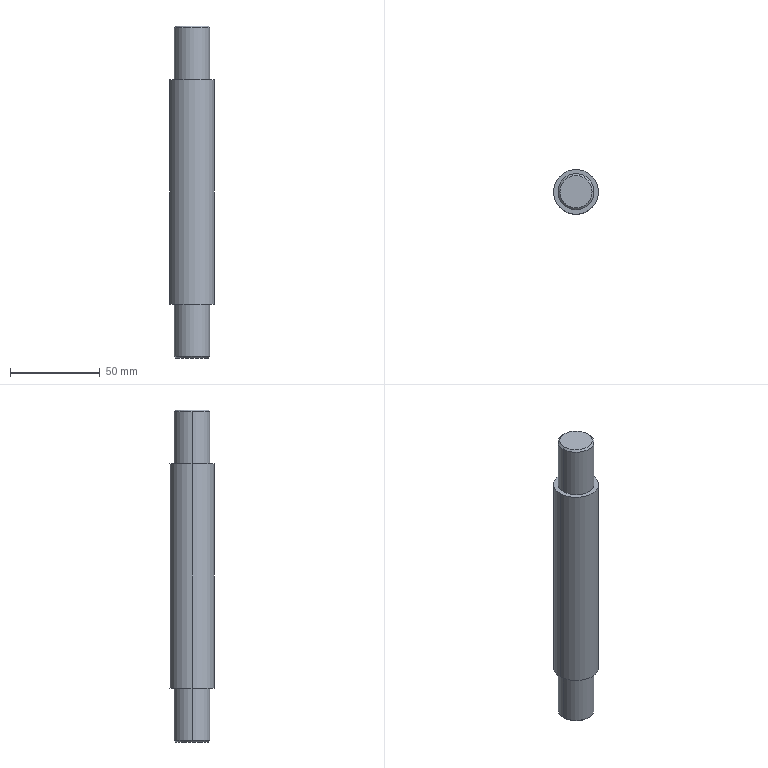Part | SolidWorks | features ICE 2, Chamfer 1, Extrusion 1 | 1 solid | 14 faces | box 25 x 25 x 185 mm | volume 80148 mm3 | cylinder 6 | cone 4 | plane 4 | commonest cylinder face diameters 20 x4 25 x2
STEP:
#1=CARTESIAN_POINT('',(-9.,0.,-92.5));
#2=VERTEX_POINT('',#1);
#3=CARTESIAN_POINT('',(9.,0.,-92.5));
#4=VERTEX_POINT('',#3);
#5=CARTESIAN_POINT('',(0.,0.,-92.5));
#6=DIRECTION('',(0.,0.,-1.));
#7=DIRECTION('',(-1.,0.,0.));
#8=AXIS2_PLACEMENT_3D('',#5,#6,#7);
#9=CIRCLE('',#8,9.);
#10=EDGE_CURVE('',#2,#4,#9,.T.);
#11=ORIENTED_EDGE('',*,*,#10,.F.);
#12=CARTESIAN_POINT('',(-10.,0.,-91.5));
#13=VERTEX_POINT('',#12);
#14=CARTESIAN_POINT('',(-9.,0.,-92.5));
#15=DIRECTION('',(-0.7071,0.,0.7071));
#16=VECTOR('',#15,1000.);
#17=LINE('',#14,#16);
#18=EDGE_CURVE('',#2,#13,#17,.T.);
#19=ORIENTED_EDGE('',*,*,#18,.T.);
#20=CARTESIAN_POINT('',(10.,0.,-91.5));
#21=VERTEX_POINT('',#20);
#22=CARTESIAN_POINT('',(0.,0.,-91.5));
#23=DIRECTION('',(0.,0.,1.));
#24=DIRECTION('',(-1.,0.,0.));
#25=AXIS2_PLACEMENT_3D('',#22,#23,#24);
#26=CIRCLE('',#25,10.);
#27=EDGE_CURVE('',#21,#13,#26,.T.);
#28=ORIENTED_EDGE('',*,*,#27,.F.);
#29=CARTESIAN_POINT('',(9.,0.,-92.5));
#30=DIRECTION('',(0.7071,0.,0.7071));
#31=VECTOR('',#30,1000.);
#32=LINE('',#29,#31);
#33=EDGE_CURVE('',#4,#21,#32,.T.);
#34=ORIENTED_EDGE('',*,*,#33,.F.);
#35=EDGE_LOOP('',(#11,#19,#28,#34));
#36=FACE_OUTER_BOUND('',#35,.T.);
#37=CARTESIAN_POINT('',(0.,0.,-92.5));
#38=DIRECTION('',(0.,0.,1.));
#39=DIRECTION('',(1.,0.,0.));
#40=AXIS2_PLACEMENT_3D('',#37,#38,#39);
#41=CONICAL_SURFACE('',#40,9.,0.7854);
#42=ADVANCED_FACE('',(#36),#41,.T.);
#43=CARTESIAN_POINT('',(9.,0.,92.5));
#44=VERTEX_POINT('',#43);
#45=CARTESIAN_POINT('',(-9.,0.,92.5));
#46=VERTEX_POINT('',#45);
#47=CARTESIAN_POINT('',(0.,0.,92.5));
#48=DIRECTION('',(0.,0.,1.));
#49=DIRECTION('',(1.,0.,0.));
#50=AXIS2_PLACEMENT_3D('',#47,#48,#49);
#51=CIRCLE('',#50,9.);
#52=EDGE_CURVE('',#44,#46,#51,.T.);
#53=ORIENTED_EDGE('',*,*,#52,.F.);
#54=CARTESIAN_POINT('',(10.,0.,91.5));
#55=VERTEX_POINT('',#54);
#56=CARTESIAN_POINT('',(9.,0.,92.5));
#57=DIRECTION('',(0.7071,0.,-0.7071));
#58=VECTOR('',#57,1000.);
#59=LINE('',#56,#58);
#60=EDGE_CURVE('',#44,#55,#59,.T.);
#61=ORIENTED_EDGE('',*,*,#60,.T.);
#62=CARTESIAN_POINT('',(-10.,0.,91.5));
#63=VERTEX_POINT('',#62);
#64=CARTESIAN_POINT('',(0.,0.,91.5));
#65=DIRECTION('',(0.,0.,-1.));
#66=DIRECTION('',(1.,0.,0.));
#67=AXIS2_PLACEMENT_3D('',#64,#65,#66);
#68=CIRCLE('',#67,10.);
#69=EDGE_CURVE('',#63,#55,#68,.T.);
#70=ORIENTED_EDGE('',*,*,#69,.F.);
#71=CARTESIAN_POINT('',(-9.,0.,92.5));
#72=DIRECTION('',(-0.7071,0.,-0.7071));
#73=VECTOR('',#72,1000.);
#74=LINE('',#71,#73);
#75=EDGE_CURVE('',#46,#63,#74,.T.);
#76=ORIENTED_EDGE('',*,*,#75,.F.);
#77=EDGE_LOOP('',(#53,#61,#70,#76));
#78=FACE_OUTER_BOUND('',#77,.T.);
#79=CARTESIAN_POINT('',(0.,0.,92.5));
#80=DIRECTION('',(0.,0.,-1.));
#81=DIRECTION('',(-1.,0.,0.));
#82=AXIS2_PLACEMENT_3D('',#79,#80,#81);
#83=CONICAL_SURFACE('',#82,9.,0.7854);
#84=ADVANCED_FACE('',(#78),#83,.T.);
#85=ORIENTED_EDGE('',*,*,#27,.T.);
#86=CARTESIAN_POINT('',(-10.,0.,-62.5));
#87=VERTEX_POINT('',#86);
#88=CARTESIAN_POINT('',(-10.,0.,-92.5));
#89=DIRECTION('',(0.,0.,1.));
#90=VECTOR('',#89,1000.);
#91=LINE('',#88,#90);
#92=EDGE_CURVE('',#13,#87,#91,.T.);
#93=ORIENTED_EDGE('',*,*,#92,.T.);
#94=CARTESIAN_POINT('',(10.,0.,-62.5));
#95=VERTEX_POINT('',#94);
#96=CARTESIAN_POINT('',(0.,0.,-62.5));
#97=DIRECTION('',(0.,0.,-1.));
#98=DIRECTION('',(-1.,0.,0.));
#99=AXIS2_PLACEMENT_3D('',#96,#97,#98);
#100=CIRCLE('',#99,10.);
#101=EDGE_CURVE('',#87,#95,#100,.T.);
#102=ORIENTED_EDGE('',*,*,#101,.T.);
#103=CARTESIAN_POINT('',(10.,0.,-92.5));
#104=DIRECTION('',(0.,0.,1.));
#105=VECTOR('',#104,1000.);
#106=LINE('',#103,#105);
#107=EDGE_CURVE('',#21,#95,#106,.T.);
#108=ORIENTED_EDGE('',*,*,#107,.F.);
#109=EDGE_LOOP('',(#85,#93,#102,#108));
#110=FACE_OUTER_BOUND('',#109,.T.);
#111=CARTESIAN_POINT('',(0.,0.,-92.5));
#112=DIRECTION('',(0.,0.,1.));
#113=DIRECTION('',(1.,0.,0.));
#114=AXIS2_PLACEMENT_3D('',#111,#112,#113);
#115=CYLINDRICAL_SURFACE('',#114,10.);
#116=ADVANCED_FACE('',(#110),#115,.T.);
#117=ORIENTED_EDGE('',*,*,#69,.T.);
#118=CARTESIAN_POINT('',(10.,0.,62.5));
#119=VERTEX_POINT('',#118);
#120=CARTESIAN_POINT('',(10.,0.,92.5));
#121=DIRECTION('',(0.,0.,-1.));
#122=VECTOR('',#121,1000.);
#123=LINE('',#120,#122);
#124=EDGE_CURVE('',#55,#119,#123,.T.);
#125=ORIENTED_EDGE('',*,*,#124,.T.);
#126=CARTESIAN_POINT('',(-10.,0.,62.5));
#127=VERTEX_POINT('',#126);
#128=CARTESIAN_POINT('',(0.,0.,62.5));
#129=DIRECTION('',(0.,0.,1.));
#130=DIRECTION('',(1.,0.,0.));
#131=AXIS2_PLACEMENT_3D('',#128,#129,#130);
#132=CIRCLE('',#131,10.);
#133=EDGE_CURVE('',#119,#127,#132,.T.);
#134=ORIENTED_EDGE('',*,*,#133,.T.);
#135=CARTESIAN_POINT('',(-10.,0.,92.5));
#136=DIRECTION('',(0.,0.,-1.));
#137=VECTOR('',#136,1000.);
#138=LINE('',#135,#137);
#139=EDGE_CURVE('',#63,#127,#138,.T.);
#140=ORIENTED_EDGE('',*,*,#139,.F.);
#141=EDGE_LOOP('',(#117,#125,#134,#140));
#142=FACE_OUTER_BOUND('',#141,.T.);
#143=CARTESIAN_POINT('',(0.,0.,92.5));
#144=DIRECTION('',(0.,0.,-1.));
#145=DIRECTION('',(-1.,0.,0.));
#146=AXIS2_PLACEMENT_3D('',#143,#144,#145);
#147=CYLINDRICAL_SURFACE('',#146,10.);
#148=ADVANCED_FACE('',(#142),#147,.T.);
#149=CARTESIAN_POINT('',(12.5,0.,62.5));
#150=VERTEX_POINT('',#149);
#151=CARTESIAN_POINT('',(-12.5,0.,62.5));
#152=VERTEX_POINT('',#151);
#153=CARTESIAN_POINT('',(0.,0.,62.5));
#154=DIRECTION('',(0.,0.,1.));
#155=DIRECTION('',(1.,0.,0.));
#156=AXIS2_PLACEMENT_3D('',#153,#154,#155);
#157=CIRCLE('',#156,12.5);
#158=EDGE_CURVE('',#150,#152,#157,.T.);
#159=ORIENTED_EDGE('',*,*,#158,.F.);
#160=CARTESIAN_POINT('',(12.5,0.,-62.5));
#161=VERTEX_POINT('',#160);
#162=CARTESIAN_POINT('',(12.5,0.,62.5));
#163=DIRECTION('',(0.,0.,-1.));
#164=VECTOR('',#163,1000.);
#165=LINE('',#162,#164);
#166=EDGE_CURVE('',#150,#161,#165,.T.);
#167=ORIENTED_EDGE('',*,*,#166,.T.);
#168=CARTESIAN_POINT('',(-12.5,0.,-62.5));
#169=VERTEX_POINT('',#168);
#170=CARTESIAN_POINT('',(0.,0.,-62.5));
#171=DIRECTION('',(0.,0.,1.));
#172=DIRECTION('',(1.,0.,0.));
#173=AXIS2_PLACEMENT_3D('',#170,#171,#172);
#174=CIRCLE('',#173,12.5);
#175=EDGE_CURVE('',#161,#169,#174,.T.);
#176=ORIENTED_EDGE('',*,*,#175,.T.);
#177=CARTESIAN_POINT('',(-12.5,0.,62.5));
#178=DIRECTION('',(0.,0.,-1.));
#179=VECTOR('',#178,1000.);
#180=LINE('',#177,#179);
#181=EDGE_CURVE('',#152,#169,#180,.T.);
#182=ORIENTED_EDGE('',*,*,#181,.F.);
#183=EDGE_LOOP('',(#159,#167,#176,#182));
#184=FACE_OUTER_BOUND('',#183,.T.);
#185=CARTESIAN_POINT('',(0.,0.,62.5));
#186=DIRECTION('',(0.,0.,-1.));
#187=DIRECTION('',(-1.,0.,0.));
#188=AXIS2_PLACEMENT_3D('',#185,#186,#187);
#189=CYLINDRICAL_SURFACE('',#188,12.5);
#190=ADVANCED_FACE('',(#184),#189,.T.);
#191=ORIENTED_EDGE('',*,*,#166,.F.);
#192=CARTESIAN_POINT('',(0.,0.,62.5));
#193=DIRECTION('',(0.,0.,1.));
#194=DIRECTION('',(1.,0.,0.));
#195=AXIS2_PLACEMENT_3D('',#192,#193,#194);
#196=CIRCLE('',#195,12.5);
#197=EDGE_CURVE('',#152,#150,#196,.T.);
#198=ORIENTED_EDGE('',*,*,#197,.F.);
#199=ORIENTED_EDGE('',*,*,#181,.T.);
#200=CARTESIAN_POINT('',(0.,0.,-62.5));
#201=DIRECTION('',(0.,0.,1.));
#202=DIRECTION('',(1.,0.,0.));
#203=AXIS2_PLACEMENT_3D('',#200,#201,#202);
#204=CIRCLE('',#203,12.5);
#205=EDGE_CURVE('',#169,#161,#204,.T.);
#206=ORIENTED_EDGE('',*,*,#205,.T.);
#207=EDGE_LOOP('',(#191,#198,#199,#206));
#208=FACE_OUTER_BOUND('',#207,.T.);
#209=CARTESIAN_POINT('',(0.,0.,62.5));
#210=DIRECTION('',(0.,0.,-1.));
#211=DIRECTION('',(-1.,0.,0.));
#212=AXIS2_PLACEMENT_3D('',#209,#210,#211);
#213=CYLINDRICAL_SURFACE('',#212,12.5);
#214=ADVANCED_FACE('',(#208),#213,.T.);
#215=CARTESIAN_POINT('',(0.,0.,62.5));
#216=DIRECTION('',(0.,0.,1.));
#217=DIRECTION('',(1.,0.,0.));
#218=AXIS2_PLACEMENT_3D('',#215,#216,#217);
#219=CIRCLE('',#218,10.);
#220=EDGE_CURVE('',#127,#119,#219,.T.);
#221=ORIENTED_EDGE('',*,*,#220,.F.);
#222=ORIENTED_EDGE('',*,*,#133,.F.);
#223=EDGE_LOOP('',(#221,#222));
#224=FACE_BOUND('',#223,.T.);
#225=ORIENTED_EDGE('',*,*,#197,.T.);
#226=ORIENTED_EDGE('',*,*,#158,.T.);
#227=EDGE_LOOP('',(#225,#226));
#228=FACE_OUTER_BOUND('',#227,.T.);
#229=CARTESIAN_POINT('',(0.,0.,62.5));
#230=DIRECTION('',(0.,0.,1.));
#231=DIRECTION('',(1.,0.,0.));
#232=AXIS2_PLACEMENT_3D('',#229,#230,#231);
#233=PLANE('',#232);
#234=ADVANCED_FACE('',(#224,#228),#233,.T.);
#235=CARTESIAN_POINT('',(0.,0.,-62.5));
#236=DIRECTION('',(0.,0.,-1.));
#237=DIRECTION('',(-1.,0.,0.));
#238=AXIS2_PLACEMENT_3D('',#235,#236,#237);
#239=CIRCLE('',#238,10.);
#240=EDGE_CURVE('',#95,#87,#239,.T.);
#241=ORIENTED_EDGE('',*,*,#240,.F.);
#242=ORIENTED_EDGE('',*,*,#101,.F.);
#243=EDGE_LOOP('',(#241,#242));
#244=FACE_BOUND('',#243,.T.);
#245=ORIENTED_EDGE('',*,*,#205,.F.);
#246=ORIENTED_EDGE('',*,*,#175,.F.);
#247=EDGE_LOOP('',(#245,#246));
#248=FACE_OUTER_BOUND('',#247,.T.);
#249=CARTESIAN_POINT('',(0.,0.,-62.5));
#250=DIRECTION('',(0.,0.,1.));
#251=DIRECTION('',(1.,0.,0.));
#252=AXIS2_PLACEMENT_3D('',#249,#250,#251);
#253=PLANE('',#252);
#254=ADVANCED_FACE('',(#244,#248),#253,.F.);
#255=ORIENTED_EDGE('',*,*,#124,.F.);
#256=CARTESIAN_POINT('',(0.,0.,91.5));
#257=DIRECTION('',(0.,0.,-1.));
#258=DIRECTION('',(1.,0.,0.));
#259=AXIS2_PLACEMENT_3D('',#256,#257,#258);
#260=CIRCLE('',#259,10.);
#261=EDGE_CURVE('',#55,#63,#260,.T.);
#262=ORIENTED_EDGE('',*,*,#261,.T.);
#263=ORIENTED_EDGE('',*,*,#139,.T.);
#264=ORIENTED_EDGE('',*,*,#220,.T.);
#265=EDGE_LOOP('',(#255,#262,#263,#264));
#266=FACE_OUTER_BOUND('',#265,.T.);
#267=CARTESIAN_POINT('',(0.,0.,92.5));
#268=DIRECTION('',(0.,0.,-1.));
#269=DIRECTION('',(-1.,0.,0.));
#270=AXIS2_PLACEMENT_3D('',#267,#268,#269);
#271=CYLINDRICAL_SURFACE('',#270,10.);
#272=ADVANCED_FACE('',(#266),#271,.T.);
#273=CARTESIAN_POINT('',(0.,0.,92.5));
#274=DIRECTION('',(0.,0.,1.));
#275=DIRECTION('',(1.,0.,0.));
#276=AXIS2_PLACEMENT_3D('',#273,#274,#275);
#277=CIRCLE('',#276,9.);
#278=EDGE_CURVE('',#46,#44,#277,.T.);
#279=ORIENTED_EDGE('',*,*,#278,.T.);
#280=ORIENTED_EDGE('',*,*,#52,.T.);
#281=EDGE_LOOP('',(#279,#280));
#282=FACE_OUTER_BOUND('',#281,.T.);
#283=CARTESIAN_POINT('',(0.,0.,92.5));
#284=DIRECTION('',(0.,0.,1.));
#285=DIRECTION('',(1.,0.,0.));
#286=AXIS2_PLACEMENT_3D('',#283,#284,#285);
#287=PLANE('',#286);
#288=ADVANCED_FACE('',(#282),#287,.T.);
#289=ORIENTED_EDGE('',*,*,#92,.F.);
#290=CARTESIAN_POINT('',(0.,0.,-91.5));
#291=DIRECTION('',(0.,0.,1.));
#292=DIRECTION('',(-1.,0.,0.));
#293=AXIS2_PLACEMENT_3D('',#290,#291,#292);
#294=CIRCLE('',#293,10.);
#295=EDGE_CURVE('',#13,#21,#294,.T.);
#296=ORIENTED_EDGE('',*,*,#295,.T.);
#297=ORIENTED_EDGE('',*,*,#107,.T.);
#298=ORIENTED_EDGE('',*,*,#240,.T.);
#299=EDGE_LOOP('',(#289,#296,#297,#298));
#300=FACE_OUTER_BOUND('',#299,.T.);
#301=CARTESIAN_POINT('',(0.,0.,-92.5));
#302=DIRECTION('',(0.,0.,1.));
#303=DIRECTION('',(1.,0.,0.));
#304=AXIS2_PLACEMENT_3D('',#301,#302,#303);
#305=CYLINDRICAL_SURFACE('',#304,10.);
#306=ADVANCED_FACE('',(#300),#305,.T.);
#307=CARTESIAN_POINT('',(0.,0.,-92.5));
#308=DIRECTION('',(0.,0.,-1.));
#309=DIRECTION('',(-1.,0.,0.));
#310=AXIS2_PLACEMENT_3D('',#307,#308,#309);
#311=CIRCLE('',#310,9.);
#312=EDGE_CURVE('',#4,#2,#311,.T.);
#313=ORIENTED_EDGE('',*,*,#312,.T.);
#314=ORIENTED_EDGE('',*,*,#10,.T.);
#315=EDGE_LOOP('',(#313,#314));
#316=FACE_OUTER_BOUND('',#315,.T.);
#317=CARTESIAN_POINT('',(0.,0.,-92.5));
#318=DIRECTION('',(0.,0.,-1.));
#319=DIRECTION('',(-1.,0.,0.));
#320=AXIS2_PLACEMENT_3D('',#317,#318,#319);
#321=PLANE('',#320);
#322=ADVANCED_FACE('',(#316),#321,.T.);
#323=ORIENTED_EDGE('',*,*,#60,.F.);
#324=ORIENTED_EDGE('',*,*,#278,.F.);
#325=ORIENTED_EDGE('',*,*,#75,.T.);
#326=ORIENTED_EDGE('',*,*,#261,.F.);
#327=EDGE_LOOP('',(#323,#324,#325,#326));
#328=FACE_OUTER_BOUND('',#327,.T.);
#329=CARTESIAN_POINT('',(0.,0.,92.5));
#330=DIRECTION('',(0.,0.,-1.));
#331=DIRECTION('',(-1.,0.,0.));
#332=AXIS2_PLACEMENT_3D('',#329,#330,#331);
#333=CONICAL_SURFACE('',#332,9.,0.7854);
#334=ADVANCED_FACE('',(#328),#333,.T.);
#335=ORIENTED_EDGE('',*,*,#18,.F.);
#336=ORIENTED_EDGE('',*,*,#312,.F.);
#337=ORIENTED_EDGE('',*,*,#33,.T.);
#338=ORIENTED_EDGE('',*,*,#295,.F.);
#339=EDGE_LOOP('',(#335,#336,#337,#338));
#340=FACE_OUTER_BOUND('',#339,.T.);
#341=CARTESIAN_POINT('',(0.,0.,-92.5));
#342=DIRECTION('',(0.,0.,1.));
#343=DIRECTION('',(1.,0.,0.));
#344=AXIS2_PLACEMENT_3D('',#341,#342,#343);
#345=CONICAL_SURFACE('',#344,9.,0.7854);
#346=ADVANCED_FACE('',(#340),#345,.T.);
#347=CLOSED_SHELL('',(#42,#84,#116,#148,#190,#214,#234,#254,#272,#288,#306,#322,#334,#346));
#348=MANIFOLD_SOLID_BREP('',#347);
#349=CARTESIAN_POINT('',(0.,0.,0.));
#350=DIRECTION('',(0.,0.,1.));
#351=DIRECTION('',(1.,0.,0.));
#352=AXIS2_PLACEMENT_3D('',#349,#350,#351);
#353=(LENGTH_UNIT()NAMED_UNIT(*)SI_UNIT(.MILLI.,.METRE.));
#354=UNCERTAINTY_MEASURE_WITH_UNIT(LENGTH_MEASURE(0.00001),#353,'','');
#355=(NAMED_UNIT(*)PLANE_ANGLE_UNIT()SI_UNIT($,.RADIAN.));
#356=(NAMED_UNIT(*)SI_UNIT($,.STERADIAN.)SOLID_ANGLE_UNIT());
#357=(GEOMETRIC_REPRESENTATION_CONTEXT(3)GLOBAL_UNCERTAINTY_ASSIGNED_CONTEXT((#354))GLOBAL_UNIT_ASSIGNED_CONTEXT((#353,#355,#356))REPRESENTATION_CONTEXT('',''));
#358=ADVANCED_BREP_SHAPE_REPRESENTATION('',(#348,#352),#357);